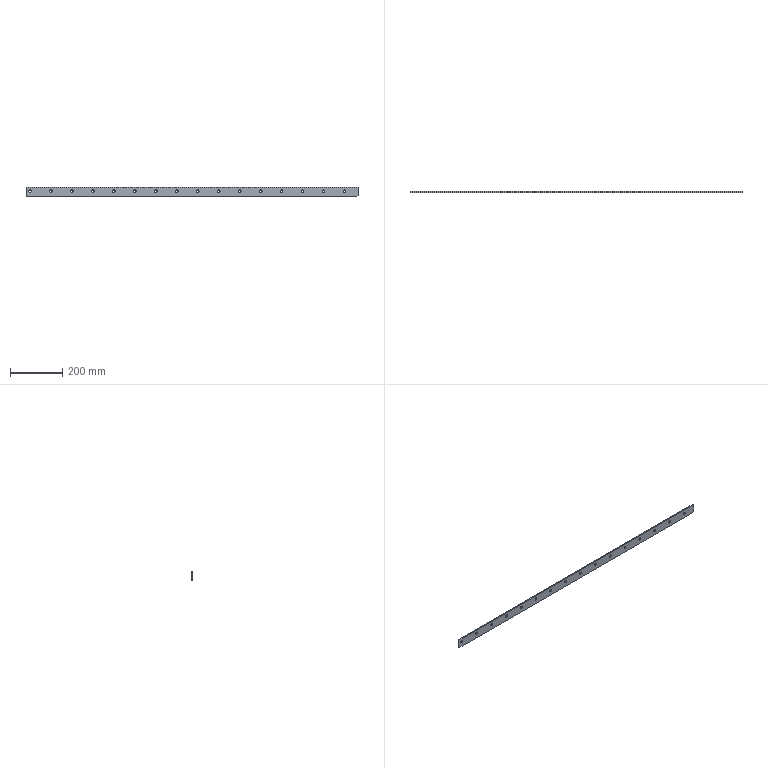Part | SolidWorks | features Chamfer 1, Extrusion 1, HoleWzd 1, LPattern 1 | 1 solid | 39 faces | box 1266 x 4 x 36 mm | volume 177227 mm3 | cylinder 32 | plane 7 | commonest cylinder face diameters 10 x32
STEP:
#1=CARTESIAN_POINT('',(-51.,0.,16.));
#2=VERTEX_POINT('',#1);
#3=CARTESIAN_POINT('',(-51.,0.,26.));
#4=VERTEX_POINT('',#3);
#5=CARTESIAN_POINT('',(-51.,0.,21.));
#6=DIRECTION('',(0.,1.,0.));
#7=DIRECTION('',(0.,0.,1.));
#8=AXIS2_PLACEMENT_3D('',#5,#6,#7);
#9=CIRCLE('',#8,5.);
#10=EDGE_CURVE('',#2,#4,#9,.T.);
#11=ORIENTED_EDGE('',*,*,#10,.F.);
#12=CARTESIAN_POINT('',(-51.,4.,16.));
#13=VERTEX_POINT('',#12);
#14=CARTESIAN_POINT('',(-51.,4.,16.));
#15=DIRECTION('',(0.,1.,0.));
#16=VECTOR('',#15,1000.);
#17=LINE('',#14,#16);
#18=EDGE_CURVE('',#2,#13,#17,.T.);
#19=ORIENTED_EDGE('',*,*,#18,.T.);
#20=CARTESIAN_POINT('',(-51.,4.,26.));
#21=VERTEX_POINT('',#20);
#22=CARTESIAN_POINT('',(-51.,4.,21.));
#23=DIRECTION('',(0.,1.,0.));
#24=DIRECTION('',(0.,0.,1.));
#25=AXIS2_PLACEMENT_3D('',#22,#23,#24);
#26=CIRCLE('',#25,5.);
#27=EDGE_CURVE('',#13,#21,#26,.T.);
#28=ORIENTED_EDGE('',*,*,#27,.T.);
#29=CARTESIAN_POINT('',(-51.,4.,26.));
#30=DIRECTION('',(0.,1.,0.));
#31=VECTOR('',#30,1000.);
#32=LINE('',#29,#31);
#33=EDGE_CURVE('',#4,#21,#32,.T.);
#34=ORIENTED_EDGE('',*,*,#33,.F.);
#35=EDGE_LOOP('',(#11,#19,#28,#34));
#36=FACE_OUTER_BOUND('',#35,.T.);
#37=CARTESIAN_POINT('',(-51.,4.,21.));
#38=DIRECTION('',(0.,1.,0.));
#39=DIRECTION('',(0.,0.,1.));
#40=AXIS2_PLACEMENT_3D('',#37,#38,#39);
#41=CYLINDRICAL_SURFACE('',#40,5.);
#42=ADVANCED_FACE('',(#36),#41,.F.);
#43=CARTESIAN_POINT('',(-131.,0.,16.));
#44=VERTEX_POINT('',#43);
#45=CARTESIAN_POINT('',(-131.,0.,26.));
#46=VERTEX_POINT('',#45);
#47=CARTESIAN_POINT('',(-131.,0.,21.));
#48=DIRECTION('',(0.,1.,0.));
#49=DIRECTION('',(0.,0.,1.));
#50=AXIS2_PLACEMENT_3D('',#47,#48,#49);
#51=CIRCLE('',#50,5.);
#52=EDGE_CURVE('',#44,#46,#51,.T.);
#53=ORIENTED_EDGE('',*,*,#52,.F.);
#54=CARTESIAN_POINT('',(-131.,4.,16.));
#55=VERTEX_POINT('',#54);
#56=CARTESIAN_POINT('',(-131.,4.,16.));
#57=DIRECTION('',(0.,1.,0.));
#58=VECTOR('',#57,1000.);
#59=LINE('',#56,#58);
#60=EDGE_CURVE('',#44,#55,#59,.T.);
#61=ORIENTED_EDGE('',*,*,#60,.T.);
#62=CARTESIAN_POINT('',(-131.,4.,26.));
#63=VERTEX_POINT('',#62);
#64=CARTESIAN_POINT('',(-131.,4.,21.));
#65=DIRECTION('',(0.,1.,0.));
#66=DIRECTION('',(0.,0.,1.));
#67=AXIS2_PLACEMENT_3D('',#64,#65,#66);
#68=CIRCLE('',#67,5.);
#69=EDGE_CURVE('',#55,#63,#68,.T.);
#70=ORIENTED_EDGE('',*,*,#69,.T.);
#71=CARTESIAN_POINT('',(-131.,4.,26.));
#72=DIRECTION('',(0.,1.,0.));
#73=VECTOR('',#72,1000.);
#74=LINE('',#71,#73);
#75=EDGE_CURVE('',#46,#63,#74,.T.);
#76=ORIENTED_EDGE('',*,*,#75,.F.);
#77=EDGE_LOOP('',(#53,#61,#70,#76));
#78=FACE_OUTER_BOUND('',#77,.T.);
#79=CARTESIAN_POINT('',(-131.,4.,21.));
#80=DIRECTION('',(0.,1.,0.));
#81=DIRECTION('',(0.,0.,1.));
#82=AXIS2_PLACEMENT_3D('',#79,#80,#81);
#83=CYLINDRICAL_SURFACE('',#82,5.);
#84=ADVANCED_FACE('',(#78),#83,.F.);
#85=CARTESIAN_POINT('',(-211.,0.,16.));
#86=VERTEX_POINT('',#85);
#87=CARTESIAN_POINT('',(-211.,0.,26.));
#88=VERTEX_POINT('',#87);
#89=CARTESIAN_POINT('',(-211.,0.,21.));
#90=DIRECTION('',(0.,1.,0.));
#91=DIRECTION('',(0.,0.,1.));
#92=AXIS2_PLACEMENT_3D('',#89,#90,#91);
#93=CIRCLE('',#92,5.);
#94=EDGE_CURVE('',#86,#88,#93,.T.);
#95=ORIENTED_EDGE('',*,*,#94,.F.);
#96=CARTESIAN_POINT('',(-211.,4.,16.));
#97=VERTEX_POINT('',#96);
#98=CARTESIAN_POINT('',(-211.,4.,16.));
#99=DIRECTION('',(0.,1.,0.));
#100=VECTOR('',#99,1000.);
#101=LINE('',#98,#100);
#102=EDGE_CURVE('',#86,#97,#101,.T.);
#103=ORIENTED_EDGE('',*,*,#102,.T.);
#104=CARTESIAN_POINT('',(-211.,4.,26.));
#105=VERTEX_POINT('',#104);
#106=CARTESIAN_POINT('',(-211.,4.,21.));
#107=DIRECTION('',(0.,1.,0.));
#108=DIRECTION('',(0.,0.,1.));
#109=AXIS2_PLACEMENT_3D('',#106,#107,#108);
#110=CIRCLE('',#109,5.);
#111=EDGE_CURVE('',#97,#105,#110,.T.);
#112=ORIENTED_EDGE('',*,*,#111,.T.);
#113=CARTESIAN_POINT('',(-211.,4.,26.));
#114=DIRECTION('',(0.,1.,0.));
#115=VECTOR('',#114,1000.);
#116=LINE('',#113,#115);
#117=EDGE_CURVE('',#88,#105,#116,.T.);
#118=ORIENTED_EDGE('',*,*,#117,.F.);
#119=EDGE_LOOP('',(#95,#103,#112,#118));
#120=FACE_OUTER_BOUND('',#119,.T.);
#121=CARTESIAN_POINT('',(-211.,4.,21.));
#122=DIRECTION('',(0.,1.,0.));
#123=DIRECTION('',(0.,0.,1.));
#124=AXIS2_PLACEMENT_3D('',#121,#122,#123);
#125=CYLINDRICAL_SURFACE('',#124,5.);
#126=ADVANCED_FACE('',(#120),#125,.F.);
#127=CARTESIAN_POINT('',(-291.,0.,16.));
#128=VERTEX_POINT('',#127);
#129=CARTESIAN_POINT('',(-291.,0.,26.));
#130=VERTEX_POINT('',#129);
#131=CARTESIAN_POINT('',(-291.,0.,21.));
#132=DIRECTION('',(0.,1.,0.));
#133=DIRECTION('',(0.,0.,1.));
#134=AXIS2_PLACEMENT_3D('',#131,#132,#133);
#135=CIRCLE('',#134,5.);
#136=EDGE_CURVE('',#128,#130,#135,.T.);
#137=ORIENTED_EDGE('',*,*,#136,.F.);
#138=CARTESIAN_POINT('',(-291.,4.,16.));
#139=VERTEX_POINT('',#138);
#140=CARTESIAN_POINT('',(-291.,4.,16.));
#141=DIRECTION('',(0.,1.,0.));
#142=VECTOR('',#141,1000.);
#143=LINE('',#140,#142);
#144=EDGE_CURVE('',#128,#139,#143,.T.);
#145=ORIENTED_EDGE('',*,*,#144,.T.);
#146=CARTESIAN_POINT('',(-291.,4.,26.));
#147=VERTEX_POINT('',#146);
#148=CARTESIAN_POINT('',(-291.,4.,21.));
#149=DIRECTION('',(0.,1.,0.));
#150=DIRECTION('',(0.,0.,1.));
#151=AXIS2_PLACEMENT_3D('',#148,#149,#150);
#152=CIRCLE('',#151,5.);
#153=EDGE_CURVE('',#139,#147,#152,.T.);
#154=ORIENTED_EDGE('',*,*,#153,.T.);
#155=CARTESIAN_POINT('',(-291.,4.,26.));
#156=DIRECTION('',(0.,1.,0.));
#157=VECTOR('',#156,1000.);
#158=LINE('',#155,#157);
#159=EDGE_CURVE('',#130,#147,#158,.T.);
#160=ORIENTED_EDGE('',*,*,#159,.F.);
#161=EDGE_LOOP('',(#137,#145,#154,#160));
#162=FACE_OUTER_BOUND('',#161,.T.);
#163=CARTESIAN_POINT('',(-291.,4.,21.));
#164=DIRECTION('',(0.,1.,0.));
#165=DIRECTION('',(0.,0.,1.));
#166=AXIS2_PLACEMENT_3D('',#163,#164,#165);
#167=CYLINDRICAL_SURFACE('',#166,5.);
#168=ADVANCED_FACE('',(#162),#167,.F.);
#169=CARTESIAN_POINT('',(-371.,0.,16.));
#170=VERTEX_POINT('',#169);
#171=CARTESIAN_POINT('',(-371.,0.,26.));
#172=VERTEX_POINT('',#171);
#173=CARTESIAN_POINT('',(-371.,0.,21.));
#174=DIRECTION('',(0.,1.,0.));
#175=DIRECTION('',(0.,0.,1.));
#176=AXIS2_PLACEMENT_3D('',#173,#174,#175);
#177=CIRCLE('',#176,5.);
#178=EDGE_CURVE('',#170,#172,#177,.T.);
#179=ORIENTED_EDGE('',*,*,#178,.F.);
#180=CARTESIAN_POINT('',(-371.,4.,16.));
#181=VERTEX_POINT('',#180);
#182=CARTESIAN_POINT('',(-371.,4.,16.));
#183=DIRECTION('',(0.,1.,0.));
#184=VECTOR('',#183,1000.);
#185=LINE('',#182,#184);
#186=EDGE_CURVE('',#170,#181,#185,.T.);
#187=ORIENTED_EDGE('',*,*,#186,.T.);
#188=CARTESIAN_POINT('',(-371.,4.,26.));
#189=VERTEX_POINT('',#188);
#190=CARTESIAN_POINT('',(-371.,4.,21.));
#191=DIRECTION('',(0.,1.,0.));
#192=DIRECTION('',(0.,0.,1.));
#193=AXIS2_PLACEMENT_3D('',#190,#191,#192);
#194=CIRCLE('',#193,5.);
#195=EDGE_CURVE('',#181,#189,#194,.T.);
#196=ORIENTED_EDGE('',*,*,#195,.T.);
#197=CARTESIAN_POINT('',(-371.,4.,26.));
#198=DIRECTION('',(0.,1.,0.));
#199=VECTOR('',#198,1000.);
#200=LINE('',#197,#199);
#201=EDGE_CURVE('',#172,#189,#200,.T.);
#202=ORIENTED_EDGE('',*,*,#201,.F.);
#203=EDGE_LOOP('',(#179,#187,#196,#202));
#204=FACE_OUTER_BOUND('',#203,.T.);
#205=CARTESIAN_POINT('',(-371.,4.,21.));
#206=DIRECTION('',(0.,1.,0.));
#207=DIRECTION('',(0.,0.,1.));
#208=AXIS2_PLACEMENT_3D('',#205,#206,#207);
#209=CYLINDRICAL_SURFACE('',#208,5.);
#210=ADVANCED_FACE('',(#204),#209,.F.);
#211=CARTESIAN_POINT('',(-451.,0.,16.));
#212=VERTEX_POINT('',#211);
#213=CARTESIAN_POINT('',(-451.,0.,26.));
#214=VERTEX_POINT('',#213);
#215=CARTESIAN_POINT('',(-451.,0.,21.));
#216=DIRECTION('',(0.,1.,0.));
#217=DIRECTION('',(0.,0.,1.));
#218=AXIS2_PLACEMENT_3D('',#215,#216,#217);
#219=CIRCLE('',#218,5.);
#220=EDGE_CURVE('',#212,#214,#219,.T.);
#221=ORIENTED_EDGE('',*,*,#220,.F.);
#222=CARTESIAN_POINT('',(-451.,4.,16.));
#223=VERTEX_POINT('',#222);
#224=CARTESIAN_POINT('',(-451.,4.,16.));
#225=DIRECTION('',(0.,1.,0.));
#226=VECTOR('',#225,1000.);
#227=LINE('',#224,#226);
#228=EDGE_CURVE('',#212,#223,#227,.T.);
#229=ORIENTED_EDGE('',*,*,#228,.T.);
#230=CARTESIAN_POINT('',(-451.,4.,26.));
#231=VERTEX_POINT('',#230);
#232=CARTESIAN_POINT('',(-451.,4.,21.));
#233=DIRECTION('',(0.,1.,0.));
#234=DIRECTION('',(0.,0.,1.));
#235=AXIS2_PLACEMENT_3D('',#232,#233,#234);
#236=CIRCLE('',#235,5.);
#237=EDGE_CURVE('',#223,#231,#236,.T.);
#238=ORIENTED_EDGE('',*,*,#237,.T.);
#239=CARTESIAN_POINT('',(-451.,4.,26.));
#240=DIRECTION('',(0.,1.,0.));
#241=VECTOR('',#240,1000.);
#242=LINE('',#239,#241);
#243=EDGE_CURVE('',#214,#231,#242,.T.);
#244=ORIENTED_EDGE('',*,*,#243,.F.);
#245=EDGE_LOOP('',(#221,#229,#238,#244));
#246=FACE_OUTER_BOUND('',#245,.T.);
#247=CARTESIAN_POINT('',(-451.,4.,21.));
#248=DIRECTION('',(0.,1.,0.));
#249=DIRECTION('',(0.,0.,1.));
#250=AXIS2_PLACEMENT_3D('',#247,#248,#249);
#251=CYLINDRICAL_SURFACE('',#250,5.);
#252=ADVANCED_FACE('',(#246),#251,.F.);
#253=CARTESIAN_POINT('',(-531.,0.,16.));
#254=VERTEX_POINT('',#253);
#255=CARTESIAN_POINT('',(-531.,0.,26.));
#256=VERTEX_POINT('',#255);
#257=CARTESIAN_POINT('',(-531.,0.,21.));
#258=DIRECTION('',(0.,1.,0.));
#259=DIRECTION('',(0.,0.,1.));
#260=AXIS2_PLACEMENT_3D('',#257,#258,#259);
#261=CIRCLE('',#260,5.);
#262=EDGE_CURVE('',#254,#256,#261,.T.);
#263=ORIENTED_EDGE('',*,*,#262,.F.);
#264=CARTESIAN_POINT('',(-531.,4.,16.));
#265=VERTEX_POINT('',#264);
#266=CARTESIAN_POINT('',(-531.,4.,16.));
#267=DIRECTION('',(0.,1.,0.));
#268=VECTOR('',#267,1000.);
#269=LINE('',#266,#268);
#270=EDGE_CURVE('',#254,#265,#269,.T.);
#271=ORIENTED_EDGE('',*,*,#270,.T.);
#272=CARTESIAN_POINT('',(-531.,4.,26.));
#273=VERTEX_POINT('',#272);
#274=CARTESIAN_POINT('',(-531.,4.,21.));
#275=DIRECTION('',(0.,1.,0.));
#276=DIRECTION('',(0.,0.,1.));
#277=AXIS2_PLACEMENT_3D('',#274,#275,#276);
#278=CIRCLE('',#277,5.);
#279=EDGE_CURVE('',#265,#273,#278,.T.);
#280=ORIENTED_EDGE('',*,*,#279,.T.);
#281=CARTESIAN_POINT('',(-531.,4.,26.));
#282=DIRECTION('',(0.,1.,0.));
#283=VECTOR('',#282,1000.);
#284=LINE('',#281,#283);
#285=EDGE_CURVE('',#256,#273,#284,.T.);
#286=ORIENTED_EDGE('',*,*,#285,.F.);
#287=EDGE_LOOP('',(#263,#271,#280,#286));
#288=FACE_OUTER_BOUND('',#287,.T.);
#289=CARTESIAN_POINT('',(-531.,4.,21.));
#290=DIRECTION('',(0.,1.,0.));
#291=DIRECTION('',(0.,0.,1.));
#292=AXIS2_PLACEMENT_3D('',#289,#290,#291);
#293=CYLINDRICAL_SURFACE('',#292,5.);
#294=ADVANCED_FACE('',(#288),#293,.F.);
#295=CARTESIAN_POINT('',(-611.,0.,16.));
#296=VERTEX_POINT('',#295);
#297=CARTESIAN_POINT('',(-611.,0.,26.));
#298=VERTEX_POINT('',#297);
#299=CARTESIAN_POINT('',(-611.,0.,21.));
#300=DIRECTION('',(0.,1.,0.));
#301=DIRECTION('',(0.,0.,1.));
#302=AXIS2_PLACEMENT_3D('',#299,#300,#301);
#303=CIRCLE('',#302,5.);
#304=EDGE_CURVE('',#296,#298,#303,.T.);
#305=ORIENTED_EDGE('',*,*,#304,.F.);
#306=CARTESIAN_POINT('',(-611.,4.,16.));
#307=VERTEX_POINT('',#306);
#308=CARTESIAN_POINT('',(-611.,4.,16.));
#309=DIRECTION('',(0.,1.,0.));
#310=VECTOR('',#309,1000.);
#311=LINE('',#308,#310);
#312=EDGE_CURVE('',#296,#307,#311,.T.);
#313=ORIENTED_EDGE('',*,*,#312,.T.);
#314=CARTESIAN_POINT('',(-611.,4.,26.));
#315=VERTEX_POINT('',#314);
#316=CARTESIAN_POINT('',(-611.,4.,21.));
#317=DIRECTION('',(0.,1.,0.));
#318=DIRECTION('',(0.,0.,1.));
#319=AXIS2_PLACEMENT_3D('',#316,#317,#318);
#320=CIRCLE('',#319,5.);
#321=EDGE_CURVE('',#307,#315,#320,.T.);
#322=ORIENTED_EDGE('',*,*,#321,.T.);
#323=CARTESIAN_POINT('',(-611.,4.,26.));
#324=DIRECTION('',(0.,1.,0.));
#325=VECTOR('',#324,1000.);
#326=LINE('',#323,#325);
#327=EDGE_CURVE('',#298,#315,#326,.T.);
#328=ORIENTED_EDGE('',*,*,#327,.F.);
#329=EDGE_LOOP('',(#305,#313,#322,#328));
#330=FACE_OUTER_BOUND('',#329,.T.);
#331=CARTESIAN_POINT('',(-611.,4.,21.));
#332=DIRECTION('',(0.,1.,0.));
#333=DIRECTION('',(0.,0.,1.));
#334=AXIS2_PLACEMENT_3D('',#331,#332,#333);
#335=CYLINDRICAL_SURFACE('',#334,5.);
#336=ADVANCED_FACE('',(#330),#335,.F.);
#337=CARTESIAN_POINT('',(-691.,0.,16.));
#338=VERTEX_POINT('',#337);
#339=CARTESIAN_POINT('',(-691.,0.,26.));
#340=VERTEX_POINT('',#339);
#341=CARTESIAN_POINT('',(-691.,0.,21.));
#342=DIRECTION('',(0.,1.,0.));
#343=DIRECTION('',(0.,0.,1.));
#344=AXIS2_PLACEMENT_3D('',#341,#342,#343);
#345=CIRCLE('',#344,5.);
#346=EDGE_CURVE('',#338,#340,#345,.T.);
#347=ORIENTED_EDGE('',*,*,#346,.F.);
#348=CARTESIAN_POINT('',(-691.,4.,16.));
#349=VERTEX_POINT('',#348);
#350=CARTESIAN_POINT('',(-691.,4.,16.));
#351=DIRECTION('',(0.,1.,0.));
#352=VECTOR('',#351,1000.);
#353=LINE('',#350,#352);
#354=EDGE_CURVE('',#338,#349,#353,.T.);
#355=ORIENTED_EDGE('',*,*,#354,.T.);
#356=CARTESIAN_POINT('',(-691.,4.,26.));
#357=VERTEX_POINT('',#356);
#358=CARTESIAN_POINT('',(-691.,4.,21.));
#359=DIRECTION('',(0.,1.,0.));
#360=DIRECTION('',(0.,0.,1.));
#361=AXIS2_PLACEMENT_3D('',#358,#359,#360);
#362=CIRCLE('',#361,5.);
#363=EDGE_CURVE('',#349,#357,#362,.T.);
#364=ORIENTED_EDGE('',*,*,#363,.T.);
#365=CARTESIAN_POINT('',(-691.,4.,26.));
#366=DIRECTION('',(0.,1.,0.));
#367=VECTOR('',#366,1000.);
#368=LINE('',#365,#367);
#369=EDGE_CURVE('',#340,#357,#368,.T.);
#370=ORIENTED_EDGE('',*,*,#369,.F.);
#371=EDGE_LOOP('',(#347,#355,#364,#370));
#372=FACE_OUTER_BOUND('',#371,.T.);
#373=CARTESIAN_POINT('',(-691.,4.,21.));
#374=DIRECTION('',(0.,1.,0.));
#375=DIRECTION('',(0.,0.,1.));
#376=AXIS2_PLACEMENT_3D('',#373,#374,#375);
#377=CYLINDRICAL_SURFACE('',#376,5.);
#378=ADVANCED_FACE('',(#372),#377,.F.);
#379=CARTESIAN_POINT('',(-771.,0.,16.));
#380=VERTEX_POINT('',#379);
#381=CARTESIAN_POINT('',(-771.,0.,26.));
#382=VERTEX_POINT('',#381);
#383=CARTESIAN_POINT('',(-771.,0.,21.));
#384=DIRECTION('',(0.,1.,0.));
#385=DIRECTION('',(0.,0.,1.));
#386=AXIS2_PLACEMENT_3D('',#383,#384,#385);
#387=CIRCLE('',#386,5.);
#388=EDGE_CURVE('',#380,#382,#387,.T.);
#389=ORIENTED_EDGE('',*,*,#388,.F.);
#390=CARTESIAN_POINT('',(-771.,4.,16.));
#391=VERTEX_POINT('',#390);
#392=CARTESIAN_POINT('',(-771.,4.,16.));
#393=DIRECTION('',(0.,1.,0.));
#394=VECTOR('',#393,1000.);
#395=LINE('',#392,#394);
#396=EDGE_CURVE('',#380,#391,#395,.T.);
#397=ORIENTED_EDGE('',*,*,#396,.T.);
#398=CARTESIAN_POINT('',(-771.,4.,26.));
#399=VERTEX_POINT('',#398);
#400=CARTESIAN_POINT('',(-771.,4.,21.));
#401=DIRECTION('',(0.,1.,0.));
#402=DIRECTION('',(0.,0.,1.));
#403=AXIS2_PLACEMENT_3D('',#400,#401,#402);
#404=CIRCLE('',#403,5.);
#405=EDGE_CURVE('',#391,#399,#404,.T.);
#406=ORIENTED_EDGE('',*,*,#405,.T.);
#407=CARTESIAN_POINT('',(-771.,4.,26.));
#408=DIRECTION('',(0.,1.,0.));
#409=VECTOR('',#408,1000.);
#410=LINE('',#407,#409);
#411=EDGE_CURVE('',#382,#399,#410,.T.);
#412=ORIENTED_EDGE('',*,*,#411,.F.);
#413=EDGE_LOOP('',(#389,#397,#406,#412));
#414=FACE_OUTER_BOUND('',#413,.T.);
#415=CARTESIAN_POINT('',(-771.,4.,21.));
#416=DIRECTION('',(0.,1.,0.));
#417=DIRECTION('',(0.,0.,1.));
#418=AXIS2_PLACEMENT_3D('',#415,#416,#417);
#419=CYLINDRICAL_SURFACE('',#418,5.);
#420=ADVANCED_FACE('',(#414),#419,.F.);
#421=CARTESIAN_POINT('',(-851.,0.,16.));
#422=VERTEX_POINT('',#421);
#423=CARTESIAN_POINT('',(-851.,0.,26.));
#424=VERTEX_POINT('',#423);
#425=CARTESIAN_POINT('',(-851.,0.,21.));
#426=DIRECTION('',(0.,1.,0.));
#427=DIRECTION('',(0.,0.,1.));
#428=AXIS2_PLACEMENT_3D('',#425,#426,#427);
#429=CIRCLE('',#428,5.);
#430=EDGE_CURVE('',#422,#424,#429,.T.);
#431=ORIENTED_EDGE('',*,*,#430,.F.);
#432=CARTESIAN_POINT('',(-851.,4.,16.));
#433=VERTEX_POINT('',#432);
#434=CARTESIAN_POINT('',(-851.,4.,16.));
#435=DIRECTION('',(0.,1.,0.));
#436=VECTOR('',#435,1000.);
#437=LINE('',#434,#436);
#438=EDGE_CURVE('',#422,#433,#437,.T.);
#439=ORIENTED_EDGE('',*,*,#438,.T.);
#440=CARTESIAN_POINT('',(-851.,4.,26.));
#441=VERTEX_POINT('',#440);
#442=CARTESIAN_POINT('',(-851.,4.,21.));
#443=DIRECTION('',(0.,1.,0.));
#444=DIRECTION('',(0.,0.,1.));
#445=AXIS2_PLACEMENT_3D('',#442,#443,#444);
#446=CIRCLE('',#445,5.);
#447=EDGE_CURVE('',#433,#441,#446,.T.);
#448=ORIENTED_EDGE('',*,*,#447,.T.);
#449=CARTESIAN_POINT('',(-851.,4.,26.));
#450=DIRECTION('',(0.,1.,0.));
#451=VECTOR('',#450,1000.);
#452=LINE('',#449,#451);
#453=EDGE_CURVE('',#424,#441,#452,.T.);
#454=ORIENTED_EDGE('',*,*,#453,.F.);
#455=EDGE_LOOP('',(#431,#439,#448,#454));
#456=FACE_OUTER_BOUND('',#455,.T.);
#457=CARTESIAN_POINT('',(-851.,4.,21.));
#458=DIRECTION('',(0.,1.,0.));
#459=DIRECTION('',(0.,0.,1.));
#460=AXIS2_PLACEMENT_3D('',#457,#458,#459);
#461=CYLINDRICAL_SURFACE('',#460,5.);
#462=ADVANCED_FACE('',(#456),#461,.F.);
#463=CARTESIAN_POINT('',(-931.,0.,16.));
#464=VERTEX_POINT('',#463);
#465=CARTESIAN_POINT('',(-931.,0.,26.));
#466=VERTEX_POINT('',#465);
#467=CARTESIAN_POINT('',(-931.,0.,21.));
#468=DIRECTION('',(0.,1.,0.));
#469=DIRECTION('',(0.,0.,1.));
#470=AXIS2_PLACEMENT_3D('',#467,#468,#469);
#471=CIRCLE('',#470,5.);
#472=EDGE_CURVE('',#464,#466,#471,.T.);
#473=ORIENTED_EDGE('',*,*,#472,.F.);
#474=CARTESIAN_POINT('',(-931.,4.,16.));
#475=VERTEX_POINT('',#474);
#476=CARTESIAN_POINT('',(-931.,4.,16.));
#477=DIRECTION('',(0.,1.,0.));
#478=VECTOR('',#477,1000.);
#479=LINE('',#476,#478);
#480=EDGE_CURVE('',#464,#475,#479,.T.);
#481=ORIENTED_EDGE('',*,*,#480,.T.);
#482=CARTESIAN_POINT('',(-931.,4.,26.));
#483=VERTEX_POINT('',#482);
#484=CARTESIAN_POINT('',(-931.,4.,21.));
#485=DIRECTION('',(0.,1.,0.));
#486=DIRECTION('',(0.,0.,1.));
#487=AXIS2_PLACEMENT_3D('',#484,#485,#486);
#488=CIRCLE('',#487,5.);
#489=EDGE_CURVE('',#475,#483,#488,.T.);
#490=ORIENTED_EDGE('',*,*,#489,.T.);
#491=CARTESIAN_POINT('',(-931.,4.,26.));
#492=DIRECTION('',(0.,1.,0.));
#493=VECTOR('',#492,1000.);
#494=LINE('',#491,#493);
#495=EDGE_CURVE('',#466,#483,#494,.T.);
#496=ORIENTED_EDGE('',*,*,#495,.F.);
#497=EDGE_LOOP('',(#473,#481,#490,#496));
#498=FACE_OUTER_BOUND('',#497,.T.);
#499=CARTESIAN_POINT('',(-931.,4.,21.));
#500=DIRECTION('',(0.,1.,0.));
#501=DIRECTION('',(0.,0.,1.));
#502=AXIS2_PLACEMENT_3D('',#499,#500,#501);
#503=CYLINDRICAL_SURFACE('',#502,5.);
#504=ADVANCED_FACE('',(#498),#503,.F.);
#505=CARTESIAN_POINT('',(-1011.,0.,16.));
#506=VERTEX_POINT('',#505);
#507=CARTESIAN_POINT('',(-1011.,0.,26.));
#508=VERTEX_POINT('',#507);
#509=CARTESIAN_POINT('',(-1011.,0.,21.));
#510=DIRECTION('',(0.,1.,0.));
#511=DIRECTION('',(0.,0.,1.));
#512=AXIS2_PLACEMENT_3D('',#509,#510,#511);
#513=CIRCLE('',#512,5.);
#514=EDGE_CURVE('',#506,#508,#513,.T.);
#515=ORIENTED_EDGE('',*,*,#514,.F.);
#516=CARTESIAN_POINT('',(-1011.,4.,16.));
#517=VERTEX_POINT('',#516);
#518=CARTESIAN_POINT('',(-1011.,4.,16.));
#519=DIRECTION('',(0.,1.,0.));
#520=VECTOR('',#519,1000.);
#521=LINE('',#518,#520);
#522=EDGE_CURVE('',#506,#517,#521,.T.);
#523=ORIENTED_EDGE('',*,*,#522,.T.);
#524=CARTESIAN_POINT('',(-1011.,4.,26.));
#525=VERTEX_POINT('',#524);
#526=CARTESIAN_POINT('',(-1011.,4.,21.));
#527=DIRECTION('',(0.,1.,0.));
#528=DIRECTION('',(0.,0.,1.));
#529=AXIS2_PLACEMENT_3D('',#526,#527,#528);
#530=CIRCLE('',#529,5.);
#531=EDGE_CURVE('',#517,#525,#530,.T.);
#532=ORIENTED_EDGE('',*,*,#531,.T.);
#533=CARTESIAN_POINT('',(-1011.,4.,26.));
#534=DIRECTION('',(0.,1.,0.));
#535=VECTOR('',#534,1000.);
#536=LINE('',#533,#535);
#537=EDGE_CURVE('',#508,#525,#536,.T.);
#538=ORIENTED_EDGE('',*,*,#537,.F.);
#539=EDGE_LOOP('',(#515,#523,#532,#538));
#540=FACE_OUTER_BOUND('',#539,.T.);
#541=CARTESIAN_POINT('',(-1011.,4.,21.));
#542=DIRECTION('',(0.,1.,0.));
#543=DIRECTION('',(0.,0.,1.));
#544=AXIS2_PLACEMENT_3D('',#541,#542,#543);
#545=CYLINDRICAL_SURFACE('',#544,5.);
#546=ADVANCED_FACE('',(#540),#545,.F.);
#547=CARTESIAN_POINT('',(-1091.,0.,16.));
#548=VERTEX_POINT('',#547);
#549=CARTESIAN_POINT('',(-1091.,0.,26.));
#550=VERTEX_POINT('',#549);
#551=CARTESIAN_POINT('',(-1091.,0.,21.));
#552=DIRECTION('',(0.,1.,0.));
#553=DIRECTION('',(0.,0.,1.));
#554=AXIS2_PLACEMENT_3D('',#551,#552,#553);
#555=CIRCLE('',#554,5.);
#556=EDGE_CURVE('',#548,#550,#555,.T.);
#557=ORIENTED_EDGE('',*,*,#556,.F.);
#558=CARTESIAN_POINT('',(-1091.,4.,16.));
#559=VERTEX_POINT('',#558);
#560=CARTESIAN_POINT('',(-1091.,4.,16.));
#561=DIRECTION('',(0.,1.,0.));
#562=VECTOR('',#561,1000.);
#563=LINE('',#560,#562);
#564=EDGE_CURVE('',#548,#559,#563,.T.);
#565=ORIENTED_EDGE('',*,*,#564,.T.);
#566=CARTESIAN_POINT('',(-1091.,4.,26.));
#567=VERTEX_POINT('',#566);
#568=CARTESIAN_POINT('',(-1091.,4.,21.));
#569=DIRECTION('',(0.,1.,0.));
#570=DIRECTION('',(0.,0.,1.));
#571=AXIS2_PLACEMENT_3D('',#568,#569,#570);
#572=CIRCLE('',#571,5.);
#573=EDGE_CURVE('',#559,#567,#572,.T.);
#574=ORIENTED_EDGE('',*,*,#573,.T.);
#575=CARTESIAN_POINT('',(-1091.,4.,26.));
#576=DIRECTION('',(0.,1.,0.));
#577=VECTOR('',#576,1000.);
#578=LINE('',#575,#577);
#579=EDGE_CURVE('',#550,#567,#578,.T.);
#580=ORIENTED_EDGE('',*,*,#579,.F.);
#581=EDGE_LOOP('',(#557,#565,#574,#580));
#582=FACE_OUTER_BOUND('',#581,.T.);
#583=CARTESIAN_POINT('',(-1091.,4.,21.));
#584=DIRECTION('',(0.,1.,0.));
#585=DIRECTION('',(0.,0.,1.));
#586=AXIS2_PLACEMENT_3D('',#583,#584,#585);
#587=CYLINDRICAL_SURFACE('',#586,5.);
#588=ADVANCED_FACE('',(#582),#587,.F.);
#589=CARTESIAN_POINT('',(-1171.,0.,16.));
#590=VERTEX_POINT('',#589);
#591=CARTESIAN_POINT('',(-1171.,0.,26.));
#592=VERTEX_POINT('',#591);
#593=CARTESIAN_POINT('',(-1171.,0.,21.));
#594=DIRECTION('',(0.,1.,0.));
#595=DIRECTION('',(0.,0.,1.));
#596=AXIS2_PLACEMENT_3D('',#593,#594,#595);
#597=CIRCLE('',#596,5.);
#598=EDGE_CURVE('',#590,#592,#597,.T.);
#599=ORIENTED_EDGE('',*,*,#598,.F.);
#600=CARTESIAN_POINT('',(-1171.,4.,16.));
#601=VERTEX_POINT('',#600);
#602=CARTESIAN_POINT('',(-1171.,4.,16.));
#603=DIRECTION('',(0.,1.,0.));
#604=VECTOR('',#603,1000.);
#605=LINE('',#602,#604);
#606=EDGE_CURVE('',#590,#601,#605,.T.);
#607=ORIENTED_EDGE('',*,*,#606,.T.);
#608=CARTESIAN_POINT('',(-1171.,4.,26.));
#609=VERTEX_POINT('',#608);
#610=CARTESIAN_POINT('',(-1171.,4.,21.));
#611=DIRECTION('',(0.,1.,0.));
#612=DIRECTION('',(0.,0.,1.));
#613=AXIS2_PLACEMENT_3D('',#610,#611,#612);
#614=CIRCLE('',#613,5.);
#615=EDGE_CURVE('',#601,#609,#614,.T.);
#616=ORIENTED_EDGE('',*,*,#615,.T.);
#617=CARTESIAN_POINT('',(-1171.,4.,26.));
#618=DIRECTION('',(0.,1.,0.));
#619=VECTOR('',#618,1000.);
#620=LINE('',#617,#619);
#621=EDGE_CURVE('',#592,#609,#620,.T.);
#622=ORIENTED_EDGE('',*,*,#621,.F.);
#623=EDGE_LOOP('',(#599,#607,#616,#622));
#624=FACE_OUTER_BOUND('',#623,.T.);
#625=CARTESIAN_POINT('',(-1171.,4.,21.));
#626=DIRECTION('',(0.,1.,0.));
#627=DIRECTION('',(0.,0.,1.));
#628=AXIS2_PLACEMENT_3D('',#625,#626,#627);
#629=CYLINDRICAL_SURFACE('',#628,5.);
#630=ADVANCED_FACE('',(#624),#629,.F.);
#631=CARTESIAN_POINT('',(-1251.,0.,16.));
#632=VERTEX_POINT('',#631);
#633=CARTESIAN_POINT('',(-1251.,0.,26.));
#634=VERTEX_POINT('',#633);
#635=CARTESIAN_POINT('',(-1251.,0.,21.));
#636=DIRECTION('',(0.,1.,0.));
#637=DIRECTION('',(0.,0.,1.));
#638=AXIS2_PLACEMENT_3D('',#635,#636,#637);
#639=CIRCLE('',#638,5.);
#640=EDGE_CURVE('',#632,#634,#639,.T.);
#641=ORIENTED_EDGE('',*,*,#640,.F.);
#642=CARTESIAN_POINT('',(-1251.,4.,16.));
#643=VERTEX_POINT('',#642);
#644=CARTESIAN_POINT('',(-1251.,4.,16.));
#645=DIRECTION('',(0.,1.,0.));
#646=VECTOR('',#645,1000.);
#647=LINE('',#644,#646);
#648=EDGE_CURVE('',#632,#643,#647,.T.);
#649=ORIENTED_EDGE('',*,*,#648,.T.);
#650=CARTESIAN_POINT('',(-1251.,4.,26.));
#651=VERTEX_POINT('',#650);
#652=CARTESIAN_POINT('',(-1251.,4.,21.));
#653=DIRECTION('',(0.,1.,0.));
#654=DIRECTION('',(0.,0.,1.));
#655=AXIS2_PLACEMENT_3D('',#652,#653,#654);
#656=CIRCLE('',#655,5.);
#657=EDGE_CURVE('',#643,#651,#656,.T.);
#658=ORIENTED_EDGE('',*,*,#657,.T.);
#659=CARTESIAN_POINT('',(-1251.,4.,26.));
#660=DIRECTION('',(0.,1.,0.));
#661=VECTOR('',#660,1000.);
#662=LINE('',#659,#661);
#663=EDGE_CURVE('',#634,#651,#662,.T.);
#664=ORIENTED_EDGE('',*,*,#663,.F.);
#665=EDGE_LOOP('',(#641,#649,#658,#664));
#666=FACE_OUTER_BOUND('',#665,.T.);
#667=CARTESIAN_POINT('',(-1251.,4.,21.));
#668=DIRECTION('',(0.,1.,0.));
#669=DIRECTION('',(0.,0.,1.));
#670=AXIS2_PLACEMENT_3D('',#667,#668,#669);
#671=CYLINDRICAL_SURFACE('',#670,5.);
#672=ADVANCED_FACE('',(#666),#671,.F.);
#673=CARTESIAN_POINT('',(-1266.,0.,0.));
#674=VERTEX_POINT('',#673);
#675=CARTESIAN_POINT('',(-1266.,0.,36.));
#676=VERTEX_POINT('',#675);
#677=CARTESIAN_POINT('',(-1266.,0.,0.));
#678=DIRECTION('',(0.,0.,1.));
#679=VECTOR('',#678,1000.);
#680=LINE('',#677,#679);
#681=EDGE_CURVE('',#674,#676,#680,.T.);
#682=ORIENTED_EDGE('',*,*,#681,.T.);
#683=CARTESIAN_POINT('',(-1266.,4.,36.));
#684=VERTEX_POINT('',#683);
#685=CARTESIAN_POINT('',(-1266.,4.,36.));
#686=DIRECTION('',(0.,-1.,0.));
#687=VECTOR('',#686,1000.);
#688=LINE('',#685,#687);
#689=EDGE_CURVE('',#684,#676,#688,.T.);
#690=ORIENTED_EDGE('',*,*,#689,.F.);
#691=CARTESIAN_POINT('',(-1266.,4.,0.));
#692=VERTEX_POINT('',#691);
#693=CARTESIAN_POINT('',(-1266.,4.,0.));
#694=DIRECTION('',(0.,0.,1.));
#695=VECTOR('',#694,1000.);
#696=LINE('',#693,#695);
#697=EDGE_CURVE('',#692,#684,#696,.T.);
#698=ORIENTED_EDGE('',*,*,#697,.F.);
#699=CARTESIAN_POINT('',(-1266.,4.,0.));
#700=DIRECTION('',(0.,-1.,0.));
#701=VECTOR('',#700,1000.);
#702=LINE('',#699,#701);
#703=EDGE_CURVE('',#692,#674,#702,.T.);
#704=ORIENTED_EDGE('',*,*,#703,.T.);
#705=EDGE_LOOP('',(#682,#690,#698,#704));
#706=FACE_OUTER_BOUND('',#705,.T.);
#707=CARTESIAN_POINT('',(-1266.,4.,0.));
#708=DIRECTION('',(1.,0.,0.));
#709=DIRECTION('',(0.,0.,-1.));
#710=AXIS2_PLACEMENT_3D('',#707,#708,#709);
#711=PLANE('',#710);
#712=ADVANCED_FACE('',(#706),#711,.F.);
#713=CARTESIAN_POINT('',(0.,0.,36.));
#714=VERTEX_POINT('',#713);
#715=CARTESIAN_POINT('',(-1266.,0.,36.));
#716=DIRECTION('',(1.,0.,0.));
#717=VECTOR('',#716,1000.);
#718=LINE('',#715,#717);
#719=EDGE_CURVE('',#676,#714,#718,.T.);
#720=ORIENTED_EDGE('',*,*,#719,.T.);
#721=CARTESIAN_POINT('',(0.,4.,36.));
#722=VERTEX_POINT('',#721);
#723=CARTESIAN_POINT('',(0.,4.,36.));
#724=DIRECTION('',(0.,-1.,0.));
#725=VECTOR('',#724,1000.);
#726=LINE('',#723,#725);
#727=EDGE_CURVE('',#722,#714,#726,.T.);
#728=ORIENTED_EDGE('',*,*,#727,.F.);
#729=CARTESIAN_POINT('',(-1266.,4.,36.));
#730=DIRECTION('',(1.,0.,0.));
#731=VECTOR('',#730,1000.);
#732=LINE('',#729,#731);
#733=EDGE_CURVE('',#684,#722,#732,.T.);
#734=ORIENTED_EDGE('',*,*,#733,.F.);
#735=ORIENTED_EDGE('',*,*,#689,.T.);
#736=EDGE_LOOP('',(#720,#728,#734,#735));
#737=FACE_OUTER_BOUND('',#736,.T.);
#738=CARTESIAN_POINT('',(-1266.,4.,36.));
#739=DIRECTION('',(0.,0.,-1.));
#740=DIRECTION('',(-1.,0.,0.));
#741=AXIS2_PLACEMENT_3D('',#738,#739,#740);
#742=PLANE('',#741);
#743=ADVANCED_FACE('',(#737),#742,.F.);
#744=CARTESIAN_POINT('',(0.,0.,5.));
#745=VERTEX_POINT('',#744);
#746=CARTESIAN_POINT('',(0.,0.,0.));
#747=DIRECTION('',(0.,0.,-1.));
#748=VECTOR('',#747,1000.);
#749=LINE('',#746,#748);
#750=EDGE_CURVE('',#714,#745,#749,.T.);
#751=ORIENTED_EDGE('',*,*,#750,.T.);
#752=CARTESIAN_POINT('',(0.,4.,5.));
#753=VERTEX_POINT('',#752);
#754=CARTESIAN_POINT('',(0.,4.,5.));
#755=DIRECTION('',(0.,1.,0.));
#756=VECTOR('',#755,1000.);
#757=LINE('',#754,#756);
#758=EDGE_CURVE('',#745,#753,#757,.T.);
#759=ORIENTED_EDGE('',*,*,#758,.T.);
#760=CARTESIAN_POINT('',(0.,4.,0.));
#761=DIRECTION('',(0.,0.,-1.));
#762=VECTOR('',#761,1000.);
#763=LINE('',#760,#762);
#764=EDGE_CURVE('',#722,#753,#763,.T.);
#765=ORIENTED_EDGE('',*,*,#764,.F.);
#766=ORIENTED_EDGE('',*,*,#727,.T.);
#767=EDGE_LOOP('',(#751,#759,#765,#766));
#768=FACE_OUTER_BOUND('',#767,.T.);
#769=CARTESIAN_POINT('',(0.,4.,0.));
#770=DIRECTION('',(-1.,0.,0.));
#771=DIRECTION('',(0.,0.,1.));
#772=AXIS2_PLACEMENT_3D('',#769,#770,#771);
#773=PLANE('',#772);
#774=ADVANCED_FACE('',(#768),#773,.F.);
#775=CARTESIAN_POINT('',(-5.,4.,0.));
#776=VERTEX_POINT('',#775);
#777=CARTESIAN_POINT('',(-1266.,4.,0.));
#778=DIRECTION('',(-1.,0.,0.));
#779=VECTOR('',#778,1000.);
#780=LINE('',#777,#779);
#781=EDGE_CURVE('',#776,#692,#780,.T.);
#782=ORIENTED_EDGE('',*,*,#781,.F.);
#783=CARTESIAN_POINT('',(-5.,0.,0.));
#784=VERTEX_POINT('',#783);
#785=CARTESIAN_POINT('',(-5.,4.,0.));
#786=DIRECTION('',(0.,-1.,0.));
#787=VECTOR('',#786,1000.);
#788=LINE('',#785,#787);
#789=EDGE_CURVE('',#776,#784,#788,.T.);
#790=ORIENTED_EDGE('',*,*,#789,.T.);
#791=CARTESIAN_POINT('',(-1266.,0.,0.));
#792=DIRECTION('',(-1.,0.,0.));
#793=VECTOR('',#792,1000.);
#794=LINE('',#791,#793);
#795=EDGE_CURVE('',#784,#674,#794,.T.);
#796=ORIENTED_EDGE('',*,*,#795,.T.);
#797=ORIENTED_EDGE('',*,*,#703,.F.);
#798=EDGE_LOOP('',(#782,#790,#796,#797));
#799=FACE_OUTER_BOUND('',#798,.T.);
#800=CARTESIAN_POINT('',(-1266.,4.,0.));
#801=DIRECTION('',(0.,0.,1.));
#802=DIRECTION('',(1.,0.,0.));
#803=AXIS2_PLACEMENT_3D('',#800,#801,#802);
#804=PLANE('',#803);
#805=ADVANCED_FACE('',(#799),#804,.F.);
#806=CARTESIAN_POINT('',(-1171.,4.,21.));
#807=DIRECTION('',(0.,1.,0.));
#808=DIRECTION('',(0.,0.,1.));
#809=AXIS2_PLACEMENT_3D('',#806,#807,#808);
#810=CIRCLE('',#809,5.);
#811=EDGE_CURVE('',#609,#601,#810,.T.);
#812=ORIENTED_EDGE('',*,*,#811,.F.);
#813=ORIENTED_EDGE('',*,*,#615,.F.);
#814=EDGE_LOOP('',(#812,#813));
#815=FACE_BOUND('',#814,.T.);
#816=CARTESIAN_POINT('',(-1251.,4.,21.));
#817=DIRECTION('',(0.,1.,0.));
#818=DIRECTION('',(0.,0.,1.));
#819=AXIS2_PLACEMENT_3D('',#816,#817,#818);
#820=CIRCLE('',#819,5.);
#821=EDGE_CURVE('',#651,#643,#820,.T.);
#822=ORIENTED_EDGE('',*,*,#821,.F.);
#823=ORIENTED_EDGE('',*,*,#657,.F.);
#824=EDGE_LOOP('',(#822,#823));
#825=FACE_BOUND('',#824,.T.);
#826=ORIENTED_EDGE('',*,*,#764,.T.);
#827=CARTESIAN_POINT('',(-617.5,4.,-612.5));
#828=DIRECTION('',(-0.7071,0.,-0.7071));
#829=VECTOR('',#828,1000.);
#830=LINE('',#827,#829);
#831=EDGE_CURVE('',#753,#776,#830,.T.);
#832=ORIENTED_EDGE('',*,*,#831,.T.);
#833=ORIENTED_EDGE('',*,*,#781,.T.);
#834=ORIENTED_EDGE('',*,*,#697,.T.);
#835=ORIENTED_EDGE('',*,*,#733,.T.);
#836=EDGE_LOOP('',(#826,#832,#833,#834,#835));
#837=FACE_OUTER_BOUND('',#836,.T.);
#838=CARTESIAN_POINT('',(-1091.,4.,21.));
#839=DIRECTION('',(0.,1.,0.));
#840=DIRECTION('',(0.,0.,1.));
#841=AXIS2_PLACEMENT_3D('',#838,#839,#840);
#842=CIRCLE('',#841,5.);
#843=EDGE_CURVE('',#567,#559,#842,.T.);
#844=ORIENTED_EDGE('',*,*,#843,.F.);
#845=ORIENTED_EDGE('',*,*,#573,.F.);
#846=EDGE_LOOP('',(#844,#845));
#847=FACE_BOUND('',#846,.T.);
#848=CARTESIAN_POINT('',(-1011.,4.,21.));
#849=DIRECTION('',(0.,1.,0.));
#850=DIRECTION('',(0.,0.,1.));
#851=AXIS2_PLACEMENT_3D('',#848,#849,#850);
#852=CIRCLE('',#851,5.);
#853=EDGE_CURVE('',#525,#517,#852,.T.);
#854=ORIENTED_EDGE('',*,*,#853,.F.);
#855=ORIENTED_EDGE('',*,*,#531,.F.);
#856=EDGE_LOOP('',(#854,#855));
#857=FACE_BOUND('',#856,.T.);
#858=CARTESIAN_POINT('',(-931.,4.,21.));
#859=DIRECTION('',(0.,1.,0.));
#860=DIRECTION('',(0.,0.,1.));
#861=AXIS2_PLACEMENT_3D('',#858,#859,#860);
#862=CIRCLE('',#861,5.);
#863=EDGE_CURVE('',#483,#475,#862,.T.);
#864=ORIENTED_EDGE('',*,*,#863,.F.);
#865=ORIENTED_EDGE('',*,*,#489,.F.);
#866=EDGE_LOOP('',(#864,#865));
#867=FACE_BOUND('',#866,.T.);
#868=CARTESIAN_POINT('',(-851.,4.,21.));
#869=DIRECTION('',(0.,1.,0.));
#870=DIRECTION('',(0.,0.,1.));
#871=AXIS2_PLACEMENT_3D('',#868,#869,#870);
#872=CIRCLE('',#871,5.);
#873=EDGE_CURVE('',#441,#433,#872,.T.);
#874=ORIENTED_EDGE('',*,*,#873,.F.);
#875=ORIENTED_EDGE('',*,*,#447,.F.);
#876=EDGE_LOOP('',(#874,#875));
#877=FACE_BOUND('',#876,.T.);
#878=CARTESIAN_POINT('',(-771.,4.,21.));
#879=DIRECTION('',(0.,1.,0.));
#880=DIRECTION('',(0.,0.,1.));
#881=AXIS2_PLACEMENT_3D('',#878,#879,#880);
#882=CIRCLE('',#881,5.);
#883=EDGE_CURVE('',#399,#391,#882,.T.);
#884=ORIENTED_EDGE('',*,*,#883,.F.);
#885=ORIENTED_EDGE('',*,*,#405,.F.);
#886=EDGE_LOOP('',(#884,#885));
#887=FACE_BOUND('',#886,.T.);
#888=CARTESIAN_POINT('',(-691.,4.,21.));
#889=DIRECTION('',(0.,1.,0.));
#890=DIRECTION('',(0.,0.,1.));
#891=AXIS2_PLACEMENT_3D('',#888,#889,#890);
#892=CIRCLE('',#891,5.);
#893=EDGE_CURVE('',#357,#349,#892,.T.);
#894=ORIENTED_EDGE('',*,*,#893,.F.);
#895=ORIENTED_EDGE('',*,*,#363,.F.);
#896=EDGE_LOOP('',(#894,#895));
#897=FACE_BOUND('',#896,.T.);
#898=CARTESIAN_POINT('',(-611.,4.,21.));
#899=DIRECTION('',(0.,1.,0.));
#900=DIRECTION('',(0.,0.,1.));
#901=AXIS2_PLACEMENT_3D('',#898,#899,#900);
#902=CIRCLE('',#901,5.);
#903=EDGE_CURVE('',#315,#307,#902,.T.);
#904=ORIENTED_EDGE('',*,*,#903,.F.);
#905=ORIENTED_EDGE('',*,*,#321,.F.);
#906=EDGE_LOOP('',(#904,#905));
#907=FACE_BOUND('',#906,.T.);
#908=CARTESIAN_POINT('',(-531.,4.,21.));
#909=DIRECTION('',(0.,1.,0.));
#910=DIRECTION('',(0.,0.,1.));
#911=AXIS2_PLACEMENT_3D('',#908,#909,#910);
#912=CIRCLE('',#911,5.);
#913=EDGE_CURVE('',#273,#265,#912,.T.);
#914=ORIENTED_EDGE('',*,*,#913,.F.);
#915=ORIENTED_EDGE('',*,*,#279,.F.);
#916=EDGE_LOOP('',(#914,#915));
#917=FACE_BOUND('',#916,.T.);
#918=CARTESIAN_POINT('',(-451.,4.,21.));
#919=DIRECTION('',(0.,1.,0.));
#920=DIRECTION('',(0.,0.,1.));
#921=AXIS2_PLACEMENT_3D('',#918,#919,#920);
#922=CIRCLE('',#921,5.);
#923=EDGE_CURVE('',#231,#223,#922,.T.);
#924=ORIENTED_EDGE('',*,*,#923,.F.);
#925=ORIENTED_EDGE('',*,*,#237,.F.);
#926=EDGE_LOOP('',(#924,#925));
#927=FACE_BOUND('',#926,.T.);
#928=CARTESIAN_POINT('',(-371.,4.,21.));
#929=DIRECTION('',(0.,1.,0.));
#930=DIRECTION('',(0.,0.,1.));
#931=AXIS2_PLACEMENT_3D('',#928,#929,#930);
#932=CIRCLE('',#931,5.);
#933=EDGE_CURVE('',#189,#181,#932,.T.);
#934=ORIENTED_EDGE('',*,*,#933,.F.);
#935=ORIENTED_EDGE('',*,*,#195,.F.);
#936=EDGE_LOOP('',(#934,#935));
#937=FACE_BOUND('',#936,.T.);
#938=CARTESIAN_POINT('',(-291.,4.,21.));
#939=DIRECTION('',(0.,1.,0.));
#940=DIRECTION('',(0.,0.,1.));
#941=AXIS2_PLACEMENT_3D('',#938,#939,#940);
#942=CIRCLE('',#941,5.);
#943=EDGE_CURVE('',#147,#139,#942,.T.);
#944=ORIENTED_EDGE('',*,*,#943,.F.);
#945=ORIENTED_EDGE('',*,*,#153,.F.);
#946=EDGE_LOOP('',(#944,#945));
#947=FACE_BOUND('',#946,.T.);
#948=CARTESIAN_POINT('',(-211.,4.,21.));
#949=DIRECTION('',(0.,1.,0.));
#950=DIRECTION('',(0.,0.,1.));
#951=AXIS2_PLACEMENT_3D('',#948,#949,#950);
#952=CIRCLE('',#951,5.);
#953=EDGE_CURVE('',#105,#97,#952,.T.);
#954=ORIENTED_EDGE('',*,*,#953,.F.);
#955=ORIENTED_EDGE('',*,*,#111,.F.);
#956=EDGE_LOOP('',(#954,#955));
#957=FACE_BOUND('',#956,.T.);
#958=CARTESIAN_POINT('',(-131.,4.,21.));
#959=DIRECTION('',(0.,1.,0.));
#960=DIRECTION('',(0.,0.,1.));
#961=AXIS2_PLACEMENT_3D('',#958,#959,#960);
#962=CIRCLE('',#961,5.);
#963=EDGE_CURVE('',#63,#55,#962,.T.);
#964=ORIENTED_EDGE('',*,*,#963,.F.);
#965=ORIENTED_EDGE('',*,*,#69,.F.);
#966=EDGE_LOOP('',(#964,#965));
#967=FACE_BOUND('',#966,.T.);
#968=CARTESIAN_POINT('',(-51.,4.,21.));
#969=DIRECTION('',(0.,1.,0.));
#970=DIRECTION('',(0.,0.,1.));
#971=AXIS2_PLACEMENT_3D('',#968,#969,#970);
#972=CIRCLE('',#971,5.);
#973=EDGE_CURVE('',#21,#13,#972,.T.);
#974=ORIENTED_EDGE('',*,*,#973,.F.);
#975=ORIENTED_EDGE('',*,*,#27,.F.);
#976=EDGE_LOOP('',(#974,#975));
#977=FACE_BOUND('',#976,.T.);
#978=CARTESIAN_POINT('',(-1266.,4.,36.));
#979=DIRECTION('',(0.,1.,0.));
#980=DIRECTION('',(0.,0.,1.));
#981=AXIS2_PLACEMENT_3D('',#978,#979,#980);
#982=PLANE('',#981);
#983=ADVANCED_FACE('',(#815,#825,#837,#847,#857,#867,#877,#887,#897,#907,#917,#927,#937,#947,#957,#967,#977),#982,.T.);
#984=CARTESIAN_POINT('',(-1171.,0.,21.));
#985=DIRECTION('',(0.,1.,0.));
#986=DIRECTION('',(0.,0.,1.));
#987=AXIS2_PLACEMENT_3D('',#984,#985,#986);
#988=CIRCLE('',#987,5.);
#989=EDGE_CURVE('',#592,#590,#988,.T.);
#990=ORIENTED_EDGE('',*,*,#989,.T.);
#991=ORIENTED_EDGE('',*,*,#598,.T.);
#992=EDGE_LOOP('',(#990,#991));
#993=FACE_BOUND('',#992,.T.);
#994=CARTESIAN_POINT('',(-1251.,0.,21.));
#995=DIRECTION('',(0.,1.,0.));
#996=DIRECTION('',(0.,0.,1.));
#997=AXIS2_PLACEMENT_3D('',#994,#995,#996);
#998=CIRCLE('',#997,5.);
#999=EDGE_CURVE('',#634,#632,#998,.T.);
#1000=ORIENTED_EDGE('',*,*,#999,.T.);
#1001=ORIENTED_EDGE('',*,*,#640,.T.);
#1002=EDGE_LOOP('',(#1000,#1001));
#1003=FACE_BOUND('',#1002,.T.);
#1004=ORIENTED_EDGE('',*,*,#795,.F.);
#1005=CARTESIAN_POINT('',(-5.,0.,0.));
#1006=DIRECTION('',(0.7071,0.,0.7071));
#1007=VECTOR('',#1006,1000.);
#1008=LINE('',#1005,#1007);
#1009=EDGE_CURVE('',#784,#745,#1008,.T.);
#1010=ORIENTED_EDGE('',*,*,#1009,.T.);
#1011=ORIENTED_EDGE('',*,*,#750,.F.);
#1012=ORIENTED_EDGE('',*,*,#719,.F.);
#1013=ORIENTED_EDGE('',*,*,#681,.F.);
#1014=EDGE_LOOP('',(#1004,#1010,#1011,#1012,#1013));
#1015=FACE_OUTER_BOUND('',#1014,.T.);
#1016=CARTESIAN_POINT('',(-1091.,0.,21.));
#1017=DIRECTION('',(0.,1.,0.));
#1018=DIRECTION('',(0.,0.,1.));
#1019=AXIS2_PLACEMENT_3D('',#1016,#1017,#1018);
#1020=CIRCLE('',#1019,5.);
#1021=EDGE_CURVE('',#550,#548,#1020,.T.);
#1022=ORIENTED_EDGE('',*,*,#1021,.T.);
#1023=ORIENTED_EDGE('',*,*,#556,.T.);
#1024=EDGE_LOOP('',(#1022,#1023));
#1025=FACE_BOUND('',#1024,.T.);
#1026=CARTESIAN_POINT('',(-1011.,0.,21.));
#1027=DIRECTION('',(0.,1.,0.));
#1028=DIRECTION('',(0.,0.,1.));
#1029=AXIS2_PLACEMENT_3D('',#1026,#1027,#1028);
#1030=CIRCLE('',#1029,5.);
#1031=EDGE_CURVE('',#508,#506,#1030,.T.);
#1032=ORIENTED_EDGE('',*,*,#1031,.T.);
#1033=ORIENTED_EDGE('',*,*,#514,.T.);
#1034=EDGE_LOOP('',(#1032,#1033));
#1035=FACE_BOUND('',#1034,.T.);
#1036=CARTESIAN_POINT('',(-931.,0.,21.));
#1037=DIRECTION('',(0.,1.,0.));
#1038=DIRECTION('',(0.,0.,1.));
#1039=AXIS2_PLACEMENT_3D('',#1036,#1037,#1038);
#1040=CIRCLE('',#1039,5.);
#1041=EDGE_CURVE('',#466,#464,#1040,.T.);
#1042=ORIENTED_EDGE('',*,*,#1041,.T.);
#1043=ORIENTED_EDGE('',*,*,#472,.T.);
#1044=EDGE_LOOP('',(#1042,#1043));
#1045=FACE_BOUND('',#1044,.T.);
#1046=CARTESIAN_POINT('',(-851.,0.,21.));
#1047=DIRECTION('',(0.,1.,0.));
#1048=DIRECTION('',(0.,0.,1.));
#1049=AXIS2_PLACEMENT_3D('',#1046,#1047,#1048);
#1050=CIRCLE('',#1049,5.);
#1051=EDGE_CURVE('',#424,#422,#1050,.T.);
#1052=ORIENTED_EDGE('',*,*,#1051,.T.);
#1053=ORIENTED_EDGE('',*,*,#430,.T.);
#1054=EDGE_LOOP('',(#1052,#1053));
#1055=FACE_BOUND('',#1054,.T.);
#1056=CARTESIAN_POINT('',(-771.,0.,21.));
#1057=DIRECTION('',(0.,1.,0.));
#1058=DIRECTION('',(0.,0.,1.));
#1059=AXIS2_PLACEMENT_3D('',#1056,#1057,#1058);
#1060=CIRCLE('',#1059,5.);
#1061=EDGE_CURVE('',#382,#380,#1060,.T.);
#1062=ORIENTED_EDGE('',*,*,#1061,.T.);
#1063=ORIENTED_EDGE('',*,*,#388,.T.);
#1064=EDGE_LOOP('',(#1062,#1063));
#1065=FACE_BOUND('',#1064,.T.);
#1066=CARTESIAN_POINT('',(-691.,0.,21.));
#1067=DIRECTION('',(0.,1.,0.));
#1068=DIRECTION('',(0.,0.,1.));
#1069=AXIS2_PLACEMENT_3D('',#1066,#1067,#1068);
#1070=CIRCLE('',#1069,5.);
#1071=EDGE_CURVE('',#340,#338,#1070,.T.);
#1072=ORIENTED_EDGE('',*,*,#1071,.T.);
#1073=ORIENTED_EDGE('',*,*,#346,.T.);
#1074=EDGE_LOOP('',(#1072,#1073));
#1075=FACE_BOUND('',#1074,.T.);
#1076=CARTESIAN_POINT('',(-611.,0.,21.));
#1077=DIRECTION('',(0.,1.,0.));
#1078=DIRECTION('',(0.,0.,1.));
#1079=AXIS2_PLACEMENT_3D('',#1076,#1077,#1078);
#1080=CIRCLE('',#1079,5.);
#1081=EDGE_CURVE('',#298,#296,#1080,.T.);
#1082=ORIENTED_EDGE('',*,*,#1081,.T.);
#1083=ORIENTED_EDGE('',*,*,#304,.T.);
#1084=EDGE_LOOP('',(#1082,#1083));
#1085=FACE_BOUND('',#1084,.T.);
#1086=CARTESIAN_POINT('',(-531.,0.,21.));
#1087=DIRECTION('',(0.,1.,0.));
#1088=DIRECTION('',(0.,0.,1.));
#1089=AXIS2_PLACEMENT_3D('',#1086,#1087,#1088);
#1090=CIRCLE('',#1089,5.);
#1091=EDGE_CURVE('',#256,#254,#1090,.T.);
#1092=ORIENTED_EDGE('',*,*,#1091,.T.);
#1093=ORIENTED_EDGE('',*,*,#262,.T.);
#1094=EDGE_LOOP('',(#1092,#1093));
#1095=FACE_BOUND('',#1094,.T.);
#1096=CARTESIAN_POINT('',(-451.,0.,21.));
#1097=DIRECTION('',(0.,1.,0.));
#1098=DIRECTION('',(0.,0.,1.));
#1099=AXIS2_PLACEMENT_3D('',#1096,#1097,#1098);
#1100=CIRCLE('',#1099,5.);
#1101=EDGE_CURVE('',#214,#212,#1100,.T.);
#1102=ORIENTED_EDGE('',*,*,#1101,.T.);
#1103=ORIENTED_EDGE('',*,*,#220,.T.);
#1104=EDGE_LOOP('',(#1102,#1103));
#1105=FACE_BOUND('',#1104,.T.);
#1106=CARTESIAN_POINT('',(-371.,0.,21.));
#1107=DIRECTION('',(0.,1.,0.));
#1108=DIRECTION('',(0.,0.,1.));
#1109=AXIS2_PLACEMENT_3D('',#1106,#1107,#1108);
#1110=CIRCLE('',#1109,5.);
#1111=EDGE_CURVE('',#172,#170,#1110,.T.);
#1112=ORIENTED_EDGE('',*,*,#1111,.T.);
#1113=ORIENTED_EDGE('',*,*,#178,.T.);
#1114=EDGE_LOOP('',(#1112,#1113));
#1115=FACE_BOUND('',#1114,.T.);
#1116=CARTESIAN_POINT('',(-291.,0.,21.));
#1117=DIRECTION('',(0.,1.,0.));
#1118=DIRECTION('',(0.,0.,1.));
#1119=AXIS2_PLACEMENT_3D('',#1116,#1117,#1118);
#1120=CIRCLE('',#1119,5.);
#1121=EDGE_CURVE('',#130,#128,#1120,.T.);
#1122=ORIENTED_EDGE('',*,*,#1121,.T.);
#1123=ORIENTED_EDGE('',*,*,#136,.T.);
#1124=EDGE_LOOP('',(#1122,#1123));
#1125=FACE_BOUND('',#1124,.T.);
#1126=CARTESIAN_POINT('',(-211.,0.,21.));
#1127=DIRECTION('',(0.,1.,0.));
#1128=DIRECTION('',(0.,0.,1.));
#1129=AXIS2_PLACEMENT_3D('',#1126,#1127,#1128);
#1130=CIRCLE('',#1129,5.);
#1131=EDGE_CURVE('',#88,#86,#1130,.T.);
#1132=ORIENTED_EDGE('',*,*,#1131,.T.);
#1133=ORIENTED_EDGE('',*,*,#94,.T.);
#1134=EDGE_LOOP('',(#1132,#1133));
#1135=FACE_BOUND('',#1134,.T.);
#1136=CARTESIAN_POINT('',(-131.,0.,21.));
#1137=DIRECTION('',(0.,1.,0.));
#1138=DIRECTION('',(0.,0.,1.));
#1139=AXIS2_PLACEMENT_3D('',#1136,#1137,#1138);
#1140=CIRCLE('',#1139,5.);
#1141=EDGE_CURVE('',#46,#44,#1140,.T.);
#1142=ORIENTED_EDGE('',*,*,#1141,.T.);
#1143=ORIENTED_EDGE('',*,*,#52,.T.);
#1144=EDGE_LOOP('',(#1142,#1143));
#1145=FACE_BOUND('',#1144,.T.);
#1146=CARTESIAN_POINT('',(-51.,0.,21.));
#1147=DIRECTION('',(0.,1.,0.));
#1148=DIRECTION('',(0.,0.,1.));
#1149=AXIS2_PLACEMENT_3D('',#1146,#1147,#1148);
#1150=CIRCLE('',#1149,5.);
#1151=EDGE_CURVE('',#4,#2,#1150,.T.);
#1152=ORIENTED_EDGE('',*,*,#1151,.T.);
#1153=ORIENTED_EDGE('',*,*,#10,.T.);
#1154=EDGE_LOOP('',(#1152,#1153));
#1155=FACE_BOUND('',#1154,.T.);
#1156=CARTESIAN_POINT('',(-1266.,0.,36.));
#1157=DIRECTION('',(0.,1.,0.));
#1158=DIRECTION('',(0.,0.,1.));
#1159=AXIS2_PLACEMENT_3D('',#1156,#1157,#1158);
#1160=PLANE('',#1159);
#1161=ADVANCED_FACE('',(#993,#1003,#1015,#1025,#1035,#1045,#1055,#1065,#1075,#1085,#1095,#1105,#1115,#1125,#1135,#1145,#1155),#1160,.F.);
#1162=ORIENTED_EDGE('',*,*,#831,.F.);
#1163=ORIENTED_EDGE('',*,*,#758,.F.);
#1164=ORIENTED_EDGE('',*,*,#1009,.F.);
#1165=ORIENTED_EDGE('',*,*,#789,.F.);
#1166=EDGE_LOOP('',(#1162,#1163,#1164,#1165));
#1167=FACE_OUTER_BOUND('',#1166,.T.);
#1168=CARTESIAN_POINT('',(-5.,4.,0.));
#1169=DIRECTION('',(-0.7071,0.,0.7071));
#1170=DIRECTION('',(0.7071,0.,0.7071));
#1171=AXIS2_PLACEMENT_3D('',#1168,#1169,#1170);
#1172=PLANE('',#1171);
#1173=ADVANCED_FACE('',(#1167),#1172,.F.);
#1174=ORIENTED_EDGE('',*,*,#648,.F.);
#1175=ORIENTED_EDGE('',*,*,#999,.F.);
#1176=ORIENTED_EDGE('',*,*,#663,.T.);
#1177=ORIENTED_EDGE('',*,*,#821,.T.);
#1178=EDGE_LOOP('',(#1174,#1175,#1176,#1177));
#1179=FACE_OUTER_BOUND('',#1178,.T.);
#1180=CARTESIAN_POINT('',(-1251.,4.,21.));
#1181=DIRECTION('',(0.,1.,0.));
#1182=DIRECTION('',(0.,0.,1.));
#1183=AXIS2_PLACEMENT_3D('',#1180,#1181,#1182);
#1184=CYLINDRICAL_SURFACE('',#1183,5.);
#1185=ADVANCED_FACE('',(#1179),#1184,.F.);
#1186=ORIENTED_EDGE('',*,*,#606,.F.);
#1187=ORIENTED_EDGE('',*,*,#989,.F.);
#1188=ORIENTED_EDGE('',*,*,#621,.T.);
#1189=ORIENTED_EDGE('',*,*,#811,.T.);
#1190=EDGE_LOOP('',(#1186,#1187,#1188,#1189));
#1191=FACE_OUTER_BOUND('',#1190,.T.);
#1192=CARTESIAN_POINT('',(-1171.,4.,21.));
#1193=DIRECTION('',(0.,1.,0.));
#1194=DIRECTION('',(0.,0.,1.));
#1195=AXIS2_PLACEMENT_3D('',#1192,#1193,#1194);
#1196=CYLINDRICAL_SURFACE('',#1195,5.);
#1197=ADVANCED_FACE('',(#1191),#1196,.F.);
#1198=ORIENTED_EDGE('',*,*,#564,.F.);
#1199=ORIENTED_EDGE('',*,*,#1021,.F.);
#1200=ORIENTED_EDGE('',*,*,#579,.T.);
#1201=ORIENTED_EDGE('',*,*,#843,.T.);
#1202=EDGE_LOOP('',(#1198,#1199,#1200,#1201));
#1203=FACE_OUTER_BOUND('',#1202,.T.);
#1204=CARTESIAN_POINT('',(-1091.,4.,21.));
#1205=DIRECTION('',(0.,1.,0.));
#1206=DIRECTION('',(0.,0.,1.));
#1207=AXIS2_PLACEMENT_3D('',#1204,#1205,#1206);
#1208=CYLINDRICAL_SURFACE('',#1207,5.);
#1209=ADVANCED_FACE('',(#1203),#1208,.F.);
#1210=ORIENTED_EDGE('',*,*,#522,.F.);
#1211=ORIENTED_EDGE('',*,*,#1031,.F.);
#1212=ORIENTED_EDGE('',*,*,#537,.T.);
#1213=ORIENTED_EDGE('',*,*,#853,.T.);
#1214=EDGE_LOOP('',(#1210,#1211,#1212,#1213));
#1215=FACE_OUTER_BOUND('',#1214,.T.);
#1216=CARTESIAN_POINT('',(-1011.,4.,21.));
#1217=DIRECTION('',(0.,1.,0.));
#1218=DIRECTION('',(0.,0.,1.));
#1219=AXIS2_PLACEMENT_3D('',#1216,#1217,#1218);
#1220=CYLINDRICAL_SURFACE('',#1219,5.);
#1221=ADVANCED_FACE('',(#1215),#1220,.F.);
#1222=ORIENTED_EDGE('',*,*,#480,.F.);
#1223=ORIENTED_EDGE('',*,*,#1041,.F.);
#1224=ORIENTED_EDGE('',*,*,#495,.T.);
#1225=ORIENTED_EDGE('',*,*,#863,.T.);
#1226=EDGE_LOOP('',(#1222,#1223,#1224,#1225));
#1227=FACE_OUTER_BOUND('',#1226,.T.);
#1228=CARTESIAN_POINT('',(-931.,4.,21.));
#1229=DIRECTION('',(0.,1.,0.));
#1230=DIRECTION('',(0.,0.,1.));
#1231=AXIS2_PLACEMENT_3D('',#1228,#1229,#1230);
#1232=CYLINDRICAL_SURFACE('',#1231,5.);
#1233=ADVANCED_FACE('',(#1227),#1232,.F.);
#1234=ORIENTED_EDGE('',*,*,#438,.F.);
#1235=ORIENTED_EDGE('',*,*,#1051,.F.);
#1236=ORIENTED_EDGE('',*,*,#453,.T.);
#1237=ORIENTED_EDGE('',*,*,#873,.T.);
#1238=EDGE_LOOP('',(#1234,#1235,#1236,#1237));
#1239=FACE_OUTER_BOUND('',#1238,.T.);
#1240=CARTESIAN_POINT('',(-851.,4.,21.));
#1241=DIRECTION('',(0.,1.,0.));
#1242=DIRECTION('',(0.,0.,1.));
#1243=AXIS2_PLACEMENT_3D('',#1240,#1241,#1242);
#1244=CYLINDRICAL_SURFACE('',#1243,5.);
#1245=ADVANCED_FACE('',(#1239),#1244,.F.);
#1246=ORIENTED_EDGE('',*,*,#396,.F.);
#1247=ORIENTED_EDGE('',*,*,#1061,.F.);
#1248=ORIENTED_EDGE('',*,*,#411,.T.);
#1249=ORIENTED_EDGE('',*,*,#883,.T.);
#1250=EDGE_LOOP('',(#1246,#1247,#1248,#1249));
#1251=FACE_OUTER_BOUND('',#1250,.T.);
#1252=CARTESIAN_POINT('',(-771.,4.,21.));
#1253=DIRECTION('',(0.,1.,0.));
#1254=DIRECTION('',(0.,0.,1.));
#1255=AXIS2_PLACEMENT_3D('',#1252,#1253,#1254);
#1256=CYLINDRICAL_SURFACE('',#1255,5.);
#1257=ADVANCED_FACE('',(#1251),#1256,.F.);
#1258=ORIENTED_EDGE('',*,*,#354,.F.);
#1259=ORIENTED_EDGE('',*,*,#1071,.F.);
#1260=ORIENTED_EDGE('',*,*,#369,.T.);
#1261=ORIENTED_EDGE('',*,*,#893,.T.);
#1262=EDGE_LOOP('',(#1258,#1259,#1260,#1261));
#1263=FACE_OUTER_BOUND('',#1262,.T.);
#1264=CARTESIAN_POINT('',(-691.,4.,21.));
#1265=DIRECTION('',(0.,1.,0.));
#1266=DIRECTION('',(0.,0.,1.));
#1267=AXIS2_PLACEMENT_3D('',#1264,#1265,#1266);
#1268=CYLINDRICAL_SURFACE('',#1267,5.);
#1269=ADVANCED_FACE('',(#1263),#1268,.F.);
#1270=ORIENTED_EDGE('',*,*,#312,.F.);
#1271=ORIENTED_EDGE('',*,*,#1081,.F.);
#1272=ORIENTED_EDGE('',*,*,#327,.T.);
#1273=ORIENTED_EDGE('',*,*,#903,.T.);
#1274=EDGE_LOOP('',(#1270,#1271,#1272,#1273));
#1275=FACE_OUTER_BOUND('',#1274,.T.);
#1276=CARTESIAN_POINT('',(-611.,4.,21.));
#1277=DIRECTION('',(0.,1.,0.));
#1278=DIRECTION('',(0.,0.,1.));
#1279=AXIS2_PLACEMENT_3D('',#1276,#1277,#1278);
#1280=CYLINDRICAL_SURFACE('',#1279,5.);
#1281=ADVANCED_FACE('',(#1275),#1280,.F.);
#1282=ORIENTED_EDGE('',*,*,#270,.F.);
#1283=ORIENTED_EDGE('',*,*,#1091,.F.);
#1284=ORIENTED_EDGE('',*,*,#285,.T.);
#1285=ORIENTED_EDGE('',*,*,#913,.T.);
#1286=EDGE_LOOP('',(#1282,#1283,#1284,#1285));
#1287=FACE_OUTER_BOUND('',#1286,.T.);
#1288=CARTESIAN_POINT('',(-531.,4.,21.));
#1289=DIRECTION('',(0.,1.,0.));
#1290=DIRECTION('',(0.,0.,1.));
#1291=AXIS2_PLACEMENT_3D('',#1288,#1289,#1290);
#1292=CYLINDRICAL_SURFACE('',#1291,5.);
#1293=ADVANCED_FACE('',(#1287),#1292,.F.);
#1294=ORIENTED_EDGE('',*,*,#228,.F.);
#1295=ORIENTED_EDGE('',*,*,#1101,.F.);
#1296=ORIENTED_EDGE('',*,*,#243,.T.);
#1297=ORIENTED_EDGE('',*,*,#923,.T.);
#1298=EDGE_LOOP('',(#1294,#1295,#1296,#1297));
#1299=FACE_OUTER_BOUND('',#1298,.T.);
#1300=CARTESIAN_POINT('',(-451.,4.,21.));
#1301=DIRECTION('',(0.,1.,0.));
#1302=DIRECTION('',(0.,0.,1.));
#1303=AXIS2_PLACEMENT_3D('',#1300,#1301,#1302);
#1304=CYLINDRICAL_SURFACE('',#1303,5.);
#1305=ADVANCED_FACE('',(#1299),#1304,.F.);
#1306=ORIENTED_EDGE('',*,*,#186,.F.);
#1307=ORIENTED_EDGE('',*,*,#1111,.F.);
#1308=ORIENTED_EDGE('',*,*,#201,.T.);
#1309=ORIENTED_EDGE('',*,*,#933,.T.);
#1310=EDGE_LOOP('',(#1306,#1307,#1308,#1309));
#1311=FACE_OUTER_BOUND('',#1310,.T.);
#1312=CARTESIAN_POINT('',(-371.,4.,21.));
#1313=DIRECTION('',(0.,1.,0.));
#1314=DIRECTION('',(0.,0.,1.));
#1315=AXIS2_PLACEMENT_3D('',#1312,#1313,#1314);
#1316=CYLINDRICAL_SURFACE('',#1315,5.);
#1317=ADVANCED_FACE('',(#1311),#1316,.F.);
#1318=ORIENTED_EDGE('',*,*,#144,.F.);
#1319=ORIENTED_EDGE('',*,*,#1121,.F.);
#1320=ORIENTED_EDGE('',*,*,#159,.T.);
#1321=ORIENTED_EDGE('',*,*,#943,.T.);
#1322=EDGE_LOOP('',(#1318,#1319,#1320,#1321));
#1323=FACE_OUTER_BOUND('',#1322,.T.);
#1324=CARTESIAN_POINT('',(-291.,4.,21.));
#1325=DIRECTION('',(0.,1.,0.));
#1326=DIRECTION('',(0.,0.,1.));
#1327=AXIS2_PLACEMENT_3D('',#1324,#1325,#1326);
#1328=CYLINDRICAL_SURFACE('',#1327,5.);
#1329=ADVANCED_FACE('',(#1323),#1328,.F.);
#1330=ORIENTED_EDGE('',*,*,#102,.F.);
#1331=ORIENTED_EDGE('',*,*,#1131,.F.);
#1332=ORIENTED_EDGE('',*,*,#117,.T.);
#1333=ORIENTED_EDGE('',*,*,#953,.T.);
#1334=EDGE_LOOP('',(#1330,#1331,#1332,#1333));
#1335=FACE_OUTER_BOUND('',#1334,.T.);
#1336=CARTESIAN_POINT('',(-211.,4.,21.));
#1337=DIRECTION('',(0.,1.,0.));
#1338=DIRECTION('',(0.,0.,1.));
#1339=AXIS2_PLACEMENT_3D('',#1336,#1337,#1338);
#1340=CYLINDRICAL_SURFACE('',#1339,5.);
#1341=ADVANCED_FACE('',(#1335),#1340,.F.);
#1342=ORIENTED_EDGE('',*,*,#60,.F.);
#1343=ORIENTED_EDGE('',*,*,#1141,.F.);
#1344=ORIENTED_EDGE('',*,*,#75,.T.);
#1345=ORIENTED_EDGE('',*,*,#963,.T.);
#1346=EDGE_LOOP('',(#1342,#1343,#1344,#1345));
#1347=FACE_OUTER_BOUND('',#1346,.T.);
#1348=CARTESIAN_POINT('',(-131.,4.,21.));
#1349=DIRECTION('',(0.,1.,0.));
#1350=DIRECTION('',(0.,0.,1.));
#1351=AXIS2_PLACEMENT_3D('',#1348,#1349,#1350);
#1352=CYLINDRICAL_SURFACE('',#1351,5.);
#1353=ADVANCED_FACE('',(#1347),#1352,.F.);
#1354=ORIENTED_EDGE('',*,*,#18,.F.);
#1355=ORIENTED_EDGE('',*,*,#1151,.F.);
#1356=ORIENTED_EDGE('',*,*,#33,.T.);
#1357=ORIENTED_EDGE('',*,*,#973,.T.);
#1358=EDGE_LOOP('',(#1354,#1355,#1356,#1357));
#1359=FACE_OUTER_BOUND('',#1358,.T.);
#1360=CARTESIAN_POINT('',(-51.,4.,21.));
#1361=DIRECTION('',(0.,1.,0.));
#1362=DIRECTION('',(0.,0.,1.));
#1363=AXIS2_PLACEMENT_3D('',#1360,#1361,#1362);
#1364=CYLINDRICAL_SURFACE('',#1363,5.);
#1365=ADVANCED_FACE('',(#1359),#1364,.F.);
#1366=CLOSED_SHELL('',(#42,#84,#126,#168,#210,#252,#294,#336,#378,#420,#462,#504,#546,#588,#630,#672,#712,#743,#774,#805,#983,#1161,#1173,#1185,#1197,#1209,#1221,#1233,#1245,#1257,#1269,#1281,#1293,#1305,#1317,#1329,#1341,#1353,#1365));
#1367=MANIFOLD_SOLID_BREP('',#1366);
#1368=CARTESIAN_POINT('',(0.,0.,0.));
#1369=DIRECTION('',(0.,0.,1.));
#1370=DIRECTION('',(1.,0.,0.));
#1371=AXIS2_PLACEMENT_3D('',#1368,#1369,#1370);
#1372=(LENGTH_UNIT()NAMED_UNIT(*)SI_UNIT(.MILLI.,.METRE.));
#1373=UNCERTAINTY_MEASURE_WITH_UNIT(LENGTH_MEASURE(0.00001),#1372,'','');
#1374=(NAMED_UNIT(*)PLANE_ANGLE_UNIT()SI_UNIT($,.RADIAN.));
#1375=(NAMED_UNIT(*)SI_UNIT($,.STERADIAN.)SOLID_ANGLE_UNIT());
#1376=(GEOMETRIC_REPRESENTATION_CONTEXT(3)GLOBAL_UNCERTAINTY_ASSIGNED_CONTEXT((#1373))GLOBAL_UNIT_ASSIGNED_CONTEXT((#1372,#1374,#1375))REPRESENTATION_CONTEXT('',''));
#1377=ADVANCED_BREP_SHAPE_REPRESENTATION('',(#1367,#1371),#1376);